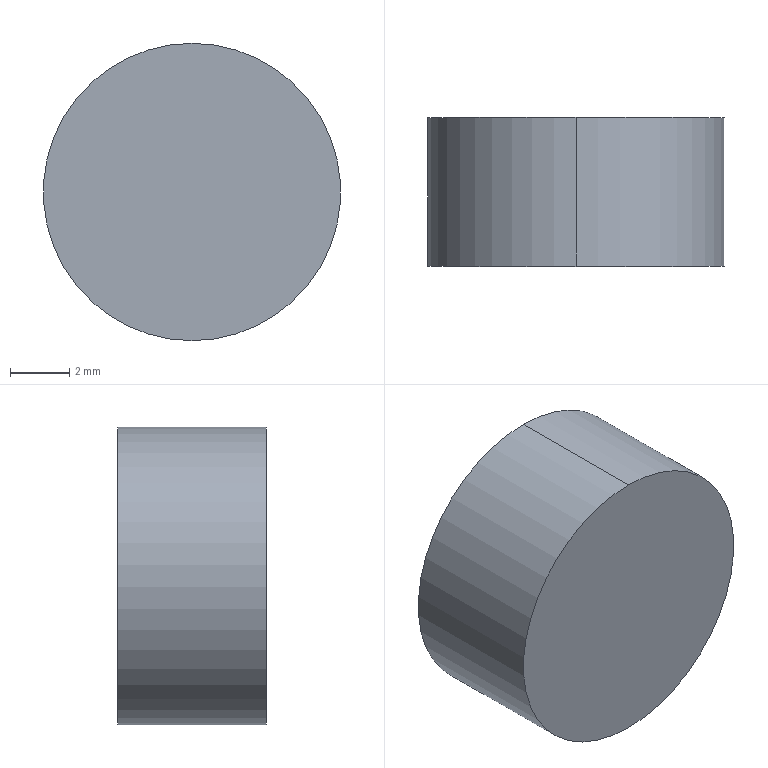Part | SolidWorks | features Extrusion 1 | 1 solid | 4 faces | box 10 x 5 x 10 mm | volume 392.699 mm3 | cylinder 2 | plane 2 | commonest cylinder face diameters 10 x2
STEP:
#1=CARTESIAN_POINT('',(0.,5.,5.));
#2=VERTEX_POINT('',#1);
#3=CARTESIAN_POINT('',(0.,5.,-5.));
#4=VERTEX_POINT('',#3);
#5=CARTESIAN_POINT('',(0.,5.,0.));
#6=DIRECTION('',(0.,1.,0.));
#7=DIRECTION('',(0.,0.,1.));
#8=AXIS2_PLACEMENT_3D('',#5,#6,#7);
#9=CIRCLE('',#8,5.);
#10=EDGE_CURVE('',#2,#4,#9,.T.);
#11=ORIENTED_EDGE('',*,*,#10,.F.);
#12=CARTESIAN_POINT('',(0.,0.,5.));
#13=VERTEX_POINT('',#12);
#14=CARTESIAN_POINT('',(0.,5.,5.));
#15=DIRECTION('',(0.,-1.,0.));
#16=VECTOR('',#15,1000.);
#17=LINE('',#14,#16);
#18=EDGE_CURVE('',#2,#13,#17,.T.);
#19=ORIENTED_EDGE('',*,*,#18,.T.);
#20=CARTESIAN_POINT('',(0.,0.,-5.));
#21=VERTEX_POINT('',#20);
#22=CARTESIAN_POINT('',(0.,0.,0.));
#23=DIRECTION('',(0.,1.,0.));
#24=DIRECTION('',(0.,0.,1.));
#25=AXIS2_PLACEMENT_3D('',#22,#23,#24);
#26=CIRCLE('',#25,5.);
#27=EDGE_CURVE('',#13,#21,#26,.T.);
#28=ORIENTED_EDGE('',*,*,#27,.T.);
#29=CARTESIAN_POINT('',(0.,5.,-5.));
#30=DIRECTION('',(0.,-1.,0.));
#31=VECTOR('',#30,1000.);
#32=LINE('',#29,#31);
#33=EDGE_CURVE('',#4,#21,#32,.T.);
#34=ORIENTED_EDGE('',*,*,#33,.F.);
#35=EDGE_LOOP('',(#11,#19,#28,#34));
#36=FACE_OUTER_BOUND('',#35,.T.);
#37=CARTESIAN_POINT('',(0.,5.,0.));
#38=DIRECTION('',(0.,-1.,0.));
#39=DIRECTION('',(0.,0.,-1.));
#40=AXIS2_PLACEMENT_3D('',#37,#38,#39);
#41=CYLINDRICAL_SURFACE('',#40,5.);
#42=ADVANCED_FACE('',(#36),#41,.T.);
#43=ORIENTED_EDGE('',*,*,#18,.F.);
#44=CARTESIAN_POINT('',(0.,5.,0.));
#45=DIRECTION('',(0.,1.,0.));
#46=DIRECTION('',(0.,0.,1.));
#47=AXIS2_PLACEMENT_3D('',#44,#45,#46);
#48=CIRCLE('',#47,5.);
#49=EDGE_CURVE('',#4,#2,#48,.T.);
#50=ORIENTED_EDGE('',*,*,#49,.F.);
#51=ORIENTED_EDGE('',*,*,#33,.T.);
#52=CARTESIAN_POINT('',(0.,0.,0.));
#53=DIRECTION('',(0.,1.,0.));
#54=DIRECTION('',(0.,0.,1.));
#55=AXIS2_PLACEMENT_3D('',#52,#53,#54);
#56=CIRCLE('',#55,5.);
#57=EDGE_CURVE('',#21,#13,#56,.T.);
#58=ORIENTED_EDGE('',*,*,#57,.T.);
#59=EDGE_LOOP('',(#43,#50,#51,#58));
#60=FACE_OUTER_BOUND('',#59,.T.);
#61=CARTESIAN_POINT('',(0.,5.,0.));
#62=DIRECTION('',(0.,-1.,0.));
#63=DIRECTION('',(0.,0.,-1.));
#64=AXIS2_PLACEMENT_3D('',#61,#62,#63);
#65=CYLINDRICAL_SURFACE('',#64,5.);
#66=ADVANCED_FACE('',(#60),#65,.T.);
#67=ORIENTED_EDGE('',*,*,#49,.T.);
#68=ORIENTED_EDGE('',*,*,#10,.T.);
#69=EDGE_LOOP('',(#67,#68));
#70=FACE_OUTER_BOUND('',#69,.T.);
#71=CARTESIAN_POINT('',(0.,5.,0.));
#72=DIRECTION('',(0.,1.,0.));
#73=DIRECTION('',(0.,0.,1.));
#74=AXIS2_PLACEMENT_3D('',#71,#72,#73);
#75=PLANE('',#74);
#76=ADVANCED_FACE('',(#70),#75,.T.);
#77=ORIENTED_EDGE('',*,*,#57,.F.);
#78=ORIENTED_EDGE('',*,*,#27,.F.);
#79=EDGE_LOOP('',(#77,#78));
#80=FACE_OUTER_BOUND('',#79,.T.);
#81=CARTESIAN_POINT('',(0.,0.,0.));
#82=DIRECTION('',(0.,1.,0.));
#83=DIRECTION('',(0.,0.,1.));
#84=AXIS2_PLACEMENT_3D('',#81,#82,#83);
#85=PLANE('',#84);
#86=ADVANCED_FACE('',(#80),#85,.F.);
#87=CLOSED_SHELL('',(#42,#66,#76,#86));
#88=MANIFOLD_SOLID_BREP('',#87);
#89=CARTESIAN_POINT('',(0.,0.,0.));
#90=DIRECTION('',(0.,0.,1.));
#91=DIRECTION('',(1.,0.,0.));
#92=AXIS2_PLACEMENT_3D('',#89,#90,#91);
#93=(LENGTH_UNIT()NAMED_UNIT(*)SI_UNIT(.MILLI.,.METRE.));
#94=UNCERTAINTY_MEASURE_WITH_UNIT(LENGTH_MEASURE(0.00001),#93,'','');
#95=(NAMED_UNIT(*)PLANE_ANGLE_UNIT()SI_UNIT($,.RADIAN.));
#96=(NAMED_UNIT(*)SI_UNIT($,.STERADIAN.)SOLID_ANGLE_UNIT());
#97=(GEOMETRIC_REPRESENTATION_CONTEXT(3)GLOBAL_UNCERTAINTY_ASSIGNED_CONTEXT((#94))GLOBAL_UNIT_ASSIGNED_CONTEXT((#93,#95,#96))REPRESENTATION_CONTEXT('',''));
#98=ADVANCED_BREP_SHAPE_REPRESENTATION('',(#88,#92),#97);